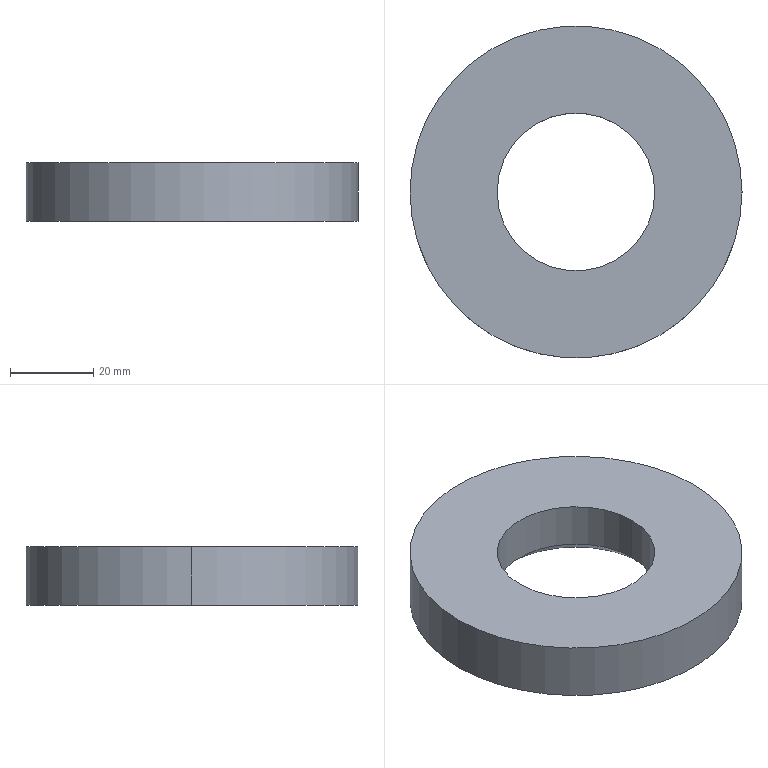Part | STEP file | 20316-2 | 1 solid | 8 faces | box 80 x 80 x 14 mm | volume 53929 mm3 | cylinder 4 | plane 2 | cone 2 | commonest cylinder face diameters 38 x2 80 x2
STEP:
#1=CARTESIAN_POINT('',(40.,0.,0.));
#2=VERTEX_POINT('',#1);
#3=CARTESIAN_POINT('',(40.,0.,14.));
#4=VERTEX_POINT('',#3);
#5=CARTESIAN_POINT('',(40.,0.,7.));
#6=DIRECTION('',(0.,0.,1.));
#7=VECTOR('',#6,1.);
#8=LINE('',#5,#7);
#9=EDGE_CURVE('',#2,#4,#8,.T.);
#10=ORIENTED_EDGE('',*,*,#9,.F.);
#11=CARTESIAN_POINT('',(-40.,0.,0.));
#12=VERTEX_POINT('',#11);
#13=CARTESIAN_POINT('',(0.,0.,0.));
#14=DIRECTION('',(0.,0.,1.));
#15=AXIS2_PLACEMENT_3D('',#13,#14,$);
#16=CIRCLE('',#15,40.);
#17=EDGE_CURVE('',#2,#12,#16,.T.);
#18=ORIENTED_EDGE('',*,*,#17,.T.);
#19=CARTESIAN_POINT('',(-40.,0.,14.));
#20=VERTEX_POINT('',#19);
#21=CARTESIAN_POINT('',(-40.,0.,7.));
#22=DIRECTION('',(0.,0.,1.));
#23=VECTOR('',#22,1.);
#24=LINE('',#21,#23);
#25=EDGE_CURVE('',#12,#20,#24,.T.);
#26=ORIENTED_EDGE('',*,*,#25,.T.);
#27=CARTESIAN_POINT('',(0.,0.,14.));
#28=DIRECTION('',(0.,0.,1.));
#29=AXIS2_PLACEMENT_3D('',#27,#28,$);
#30=CIRCLE('',#29,40.);
#31=EDGE_CURVE('',#4,#20,#30,.T.);
#32=ORIENTED_EDGE('',*,*,#31,.F.);
#33=EDGE_LOOP('',(#10,#18,#26,#32));
#34=FACE_OUTER_BOUND('',#33,.T.);
#35=CARTESIAN_POINT('',(0.,0.,7.));
#36=DIRECTION('',(0.,0.,1.));
#37=DIRECTION('',(1.,0.,0.));
#38=AXIS2_PLACEMENT_3D('',#35,#36,#37);
#39=CYLINDRICAL_SURFACE('',#38,40.);
#40=ADVANCED_FACE('',(#34),#39,.T.);
#41=ORIENTED_EDGE('',*,*,#25,.F.);
#42=CARTESIAN_POINT('',(0.,0.,0.));
#43=DIRECTION('',(0.,0.,1.));
#44=AXIS2_PLACEMENT_3D('',#42,#43,$);
#45=CIRCLE('',#44,40.);
#46=EDGE_CURVE('',#12,#2,#45,.T.);
#47=ORIENTED_EDGE('',*,*,#46,.T.);
#48=ORIENTED_EDGE('',*,*,#9,.T.);
#49=CARTESIAN_POINT('',(0.,0.,14.));
#50=DIRECTION('',(0.,0.,1.));
#51=AXIS2_PLACEMENT_3D('',#49,#50,$);
#52=CIRCLE('',#51,40.);
#53=EDGE_CURVE('',#20,#4,#52,.T.);
#54=ORIENTED_EDGE('',*,*,#53,.F.);
#55=EDGE_LOOP('',(#41,#47,#48,#54));
#56=FACE_OUTER_BOUND('',#55,.T.);
#57=ADVANCED_FACE('',(#56),#39,.T.);
#58=ORIENTED_EDGE('',*,*,#31,.T.);
#59=ORIENTED_EDGE('',*,*,#53,.T.);
#60=EDGE_LOOP('',(#58,#59));
#61=FACE_OUTER_BOUND('',#60,.T.);
#62=CARTESIAN_POINT('',(-19.,0.,14.));
#63=VERTEX_POINT('',#62);
#64=CARTESIAN_POINT('',(19.,0.,14.));
#65=VERTEX_POINT('',#64);
#66=CARTESIAN_POINT('',(0.,0.,14.));
#67=DIRECTION('',(0.,0.,1.));
#68=AXIS2_PLACEMENT_3D('',#66,#67,$);
#69=CIRCLE('',#68,19.);
#70=EDGE_CURVE('',#63,#65,#69,.T.);
#71=ORIENTED_EDGE('',*,*,#70,.F.);
#72=CARTESIAN_POINT('',(0.,0.,14.));
#73=DIRECTION('',(0.,0.,1.));
#74=AXIS2_PLACEMENT_3D('',#72,#73,$);
#75=CIRCLE('',#74,19.);
#76=EDGE_CURVE('',#65,#63,#75,.T.);
#77=ORIENTED_EDGE('',*,*,#76,.F.);
#78=EDGE_LOOP('',(#71,#77));
#79=FACE_BOUND('',#78,.T.);
#80=CARTESIAN_POINT('',(0.,0.,14.));
#81=DIRECTION('',(0.,0.,1.));
#82=DIRECTION('',(1.,0.,0.));
#83=AXIS2_PLACEMENT_3D('',#80,#81,#82);
#84=PLANE('',#83);
#85=ADVANCED_FACE('',(#61,#79),#84,.T.);
#86=CARTESIAN_POINT('',(-19.,0.,3.));
#87=VERTEX_POINT('',#86);
#88=CARTESIAN_POINT('',(19.,0.,3.));
#89=VERTEX_POINT('',#88);
#90=CARTESIAN_POINT('',(0.,0.,3.));
#91=DIRECTION('',(0.,0.,1.));
#92=AXIS2_PLACEMENT_3D('',#90,#91,$);
#93=CIRCLE('',#92,19.);
#94=EDGE_CURVE('',#87,#89,#93,.T.);
#95=ORIENTED_EDGE('',*,*,#94,.F.);
#96=CARTESIAN_POINT('',(-19.,0.,7.));
#97=DIRECTION('',(0.,0.,1.));
#98=VECTOR('',#97,1.);
#99=LINE('',#96,#98);
#100=EDGE_CURVE('',#87,#63,#99,.T.);
#101=ORIENTED_EDGE('',*,*,#100,.T.);
#102=ORIENTED_EDGE('',*,*,#70,.T.);
#103=CARTESIAN_POINT('',(19.,0.,7.));
#104=DIRECTION('',(0.,0.,1.));
#105=VECTOR('',#104,1.);
#106=LINE('',#103,#105);
#107=EDGE_CURVE('',#89,#65,#106,.T.);
#108=ORIENTED_EDGE('',*,*,#107,.F.);
#109=EDGE_LOOP('',(#95,#101,#102,#108));
#110=FACE_OUTER_BOUND('',#109,.T.);
#111=CARTESIAN_POINT('',(0.,0.,7.));
#112=DIRECTION('',(0.,0.,1.));
#113=DIRECTION('',(1.,0.,0.));
#114=AXIS2_PLACEMENT_3D('',#111,#112,#113);
#115=CYLINDRICAL_SURFACE('',#114,19.);
#116=ADVANCED_FACE('',(#110),#115,.F.);
#117=CARTESIAN_POINT('',(0.,0.,3.));
#118=DIRECTION('',(0.,0.,1.));
#119=AXIS2_PLACEMENT_3D('',#117,#118,$);
#120=CIRCLE('',#119,19.);
#121=EDGE_CURVE('',#89,#87,#120,.T.);
#122=ORIENTED_EDGE('',*,*,#121,.F.);
#123=ORIENTED_EDGE('',*,*,#107,.T.);
#124=ORIENTED_EDGE('',*,*,#76,.T.);
#125=ORIENTED_EDGE('',*,*,#100,.F.);
#126=EDGE_LOOP('',(#122,#123,#124,#125));
#127=FACE_OUTER_BOUND('',#126,.T.);
#128=ADVANCED_FACE('',(#127),#115,.F.);
#129=ORIENTED_EDGE('',*,*,#46,.F.);
#130=ORIENTED_EDGE('',*,*,#17,.F.);
#131=EDGE_LOOP('',(#129,#130));
#132=FACE_OUTER_BOUND('',#131,.T.);
#133=CARTESIAN_POINT('',(-22.,0.000000806,0.));
#134=VERTEX_POINT('',#133);
#135=CARTESIAN_POINT('',(22.,0.,0.));
#136=VERTEX_POINT('',#135);
#137=CARTESIAN_POINT('',(0.,0.,0.));
#138=DIRECTION('',(0.,0.,1.));
#139=AXIS2_PLACEMENT_3D('',#137,#138,$);
#140=CIRCLE('',#139,22.);
#141=EDGE_CURVE('',#134,#136,#140,.T.);
#142=ORIENTED_EDGE('',*,*,#141,.T.);
#143=CARTESIAN_POINT('',(0.,0.,0.));
#144=DIRECTION('',(0.,0.,1.));
#145=AXIS2_PLACEMENT_3D('',#143,#144,$);
#146=CIRCLE('',#145,22.);
#147=EDGE_CURVE('',#136,#134,#146,.T.);
#148=ORIENTED_EDGE('',*,*,#147,.T.);
#149=EDGE_LOOP('',(#142,#148));
#150=FACE_BOUND('',#149,.T.);
#151=CARTESIAN_POINT('',(0.,0.,0.));
#152=DIRECTION('',(0.,0.,1.));
#153=DIRECTION('',(1.,0.,0.));
#154=AXIS2_PLACEMENT_3D('',#151,#152,#153);
#155=PLANE('',#154);
#156=ADVANCED_FACE('',(#132,#150),#155,.F.);
#157=CARTESIAN_POINT('',(-20.5,0.,1.5));
#158=DIRECTION('',(-0.7071,0.,-0.7071));
#159=VECTOR('',#158,1.);
#160=LINE('',#157,#159);
#161=EDGE_CURVE('',#134,#87,#160,.F.);
#162=ORIENTED_EDGE('',*,*,#161,.T.);
#163=ORIENTED_EDGE('',*,*,#94,.T.);
#164=CARTESIAN_POINT('',(20.5,0.,1.5));
#165=DIRECTION('',(0.7071,0.,-0.7071));
#166=VECTOR('',#165,1.);
#167=LINE('',#164,#166);
#168=EDGE_CURVE('',#136,#89,#167,.F.);
#169=ORIENTED_EDGE('',*,*,#168,.F.);
#170=ORIENTED_EDGE('',*,*,#141,.F.);
#171=EDGE_LOOP('',(#162,#163,#169,#170));
#172=FACE_OUTER_BOUND('',#171,.T.);
#173=CARTESIAN_POINT('',(0.,0.,22.));
#174=DIRECTION('',(0.,0.,-1.));
#175=DIRECTION('',(-0.9195,0.3931,0.));
#176=AXIS2_PLACEMENT_3D('',#173,#174,#175);
#177=CONICAL_SURFACE('',#176,0.,0.7854);
#178=ADVANCED_FACE('',(#172),#177,.F.);
#179=ORIENTED_EDGE('',*,*,#168,.T.);
#180=ORIENTED_EDGE('',*,*,#121,.T.);
#181=ORIENTED_EDGE('',*,*,#161,.F.);
#182=ORIENTED_EDGE('',*,*,#147,.F.);
#183=EDGE_LOOP('',(#179,#180,#181,#182));
#184=FACE_OUTER_BOUND('',#183,.T.);
#185=CARTESIAN_POINT('',(0.,0.,22.));
#186=DIRECTION('',(0.,0.,-1.));
#187=DIRECTION('',(1.,0.,0.));
#188=AXIS2_PLACEMENT_3D('',#185,#186,#187);
#189=CONICAL_SURFACE('',#188,0.,0.7854);
#190=ADVANCED_FACE('',(#184),#189,.F.);
#191=CLOSED_SHELL('',(#40,#57,#85,#116,#128,#156,#178,#190));
#192=MANIFOLD_SOLID_BREP('',#191);
#193=(LENGTH_UNIT()NAMED_UNIT(*)SI_UNIT(.MILLI.,.METRE.));
#194=UNCERTAINTY_MEASURE_WITH_UNIT(LENGTH_MEASURE(0.005),#193,'','');
#195=(NAMED_UNIT(*)PLANE_ANGLE_UNIT()SI_UNIT($,.RADIAN.));
#196=(NAMED_UNIT(*)SI_UNIT($,.STERADIAN.)SOLID_ANGLE_UNIT());
#197=(GEOMETRIC_REPRESENTATION_CONTEXT(3)GLOBAL_UNCERTAINTY_ASSIGNED_CONTEXT((#194))GLOBAL_UNIT_ASSIGNED_CONTEXT((#193,#195,#196))REPRESENTATION_CONTEXT('',''));
#198=ADVANCED_BREP_SHAPE_REPRESENTATION('',(#192),#197);